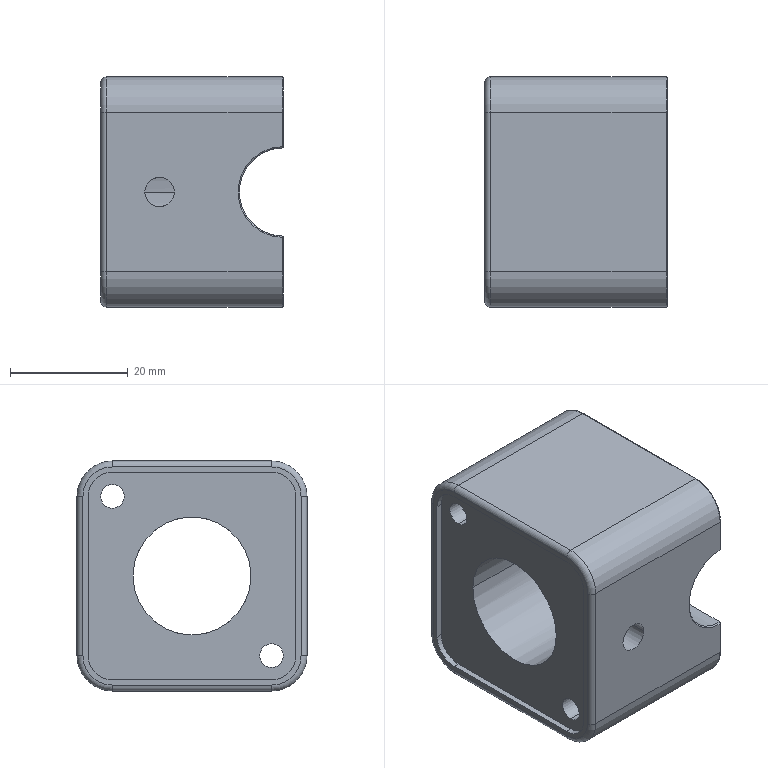Part | 1 solid | 62 faces | box 31 x 39 x 39 mm | volume 32063 mm3 | cylinder 36 | plane 16 | torus 8 | cone 2 | commonest cylinder face diameters 0.4 x6 2 x4 3.2 x4 4 x4 7.2 x4 8.2 x4